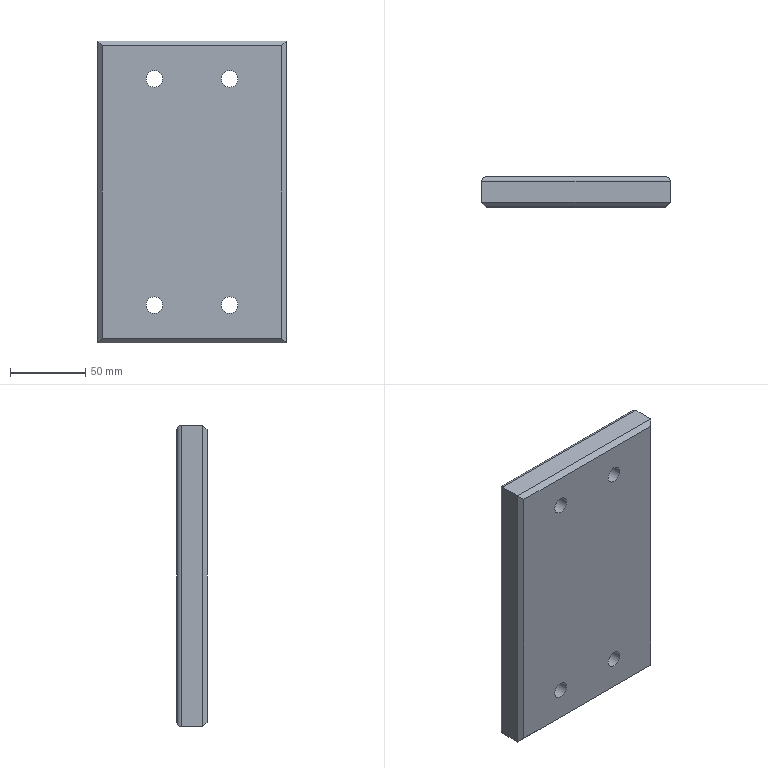Part | NX | features solid 2 | 1 solid | 26 faces | box 125 x 20 x 200 mm | volume 481280 mm3 | plane 14 | cylinder 12 | commonest cylinder face diameters 6 x4 11 x4 17.5 x4
STEP:
#1=CARTESIAN_POINT('',(-972.5,528.,-185.));
#2=VERTEX_POINT('',#1);
#3=CARTESIAN_POINT('',(-972.5,542.,-185.));
#4=VERTEX_POINT('',#3);
#5=CARTESIAN_POINT('',(-972.5,525.,-185.));
#6=DIRECTION('',(0.,1.,0.));
#7=VECTOR('',#6,1000.);
#8=LINE('',#5,#7);
#9=EDGE_CURVE('',#2,#4,#8,.T.);
#10=ORIENTED_EDGE('',*,*,#9,.F.);
#11=CARTESIAN_POINT('',(-1097.5,528.,-185.));
#12=VERTEX_POINT('',#11);
#13=CARTESIAN_POINT('',(-1097.5,528.,-185.));
#14=DIRECTION('',(-1.,0.,0.));
#15=VECTOR('',#14,1000.);
#16=LINE('',#13,#15);
#17=EDGE_CURVE('',#2,#12,#16,.T.);
#18=ORIENTED_EDGE('',*,*,#17,.T.);
#19=CARTESIAN_POINT('',(-1097.5,542.,-185.));
#20=VERTEX_POINT('',#19);
#21=CARTESIAN_POINT('',(-1097.5,525.,-185.));
#22=DIRECTION('',(0.,1.,0.));
#23=VECTOR('',#22,1000.);
#24=LINE('',#21,#23);
#25=EDGE_CURVE('',#12,#20,#24,.T.);
#26=ORIENTED_EDGE('',*,*,#25,.T.);
#27=CARTESIAN_POINT('',(-972.5,542.,-185.));
#28=DIRECTION('',(1.,0.,0.));
#29=VECTOR('',#28,1000.);
#30=LINE('',#27,#29);
#31=EDGE_CURVE('',#20,#4,#30,.T.);
#32=ORIENTED_EDGE('',*,*,#31,.T.);
#33=EDGE_LOOP('',(#10,#18,#26,#32));
#34=FACE_BOUND('',#33,.T.);
#35=CARTESIAN_POINT('',(-1097.5,525.,-185.));
#36=DIRECTION('',(0.,0.,1.));
#37=DIRECTION('',(-1.,0.,0.));
#38=AXIS2_PLACEMENT_3D('',#35,#36,#37);
#39=PLANE('',#38);
#40=ADVANCED_FACE('',(#34),#39,.F.);
#41=CARTESIAN_POINT('',(-972.5,528.,15.));
#42=VERTEX_POINT('',#41);
#43=CARTESIAN_POINT('',(-972.5,542.,15.));
#44=VERTEX_POINT('',#43);
#45=CARTESIAN_POINT('',(-972.5,525.,15.));
#46=DIRECTION('',(0.,1.,0.));
#47=VECTOR('',#46,1000.);
#48=LINE('',#45,#47);
#49=EDGE_CURVE('',#42,#44,#48,.T.);
#50=ORIENTED_EDGE('',*,*,#49,.F.);
#51=CARTESIAN_POINT('',(-972.5,528.,-185.));
#52=DIRECTION('',(0.,0.,-1.));
#53=VECTOR('',#52,1000.);
#54=LINE('',#51,#53);
#55=EDGE_CURVE('',#42,#2,#54,.T.);
#56=ORIENTED_EDGE('',*,*,#55,.T.);
#57=ORIENTED_EDGE('',*,*,#9,.T.);
#58=CARTESIAN_POINT('',(-972.5,542.,15.));
#59=DIRECTION('',(0.,0.,1.));
#60=VECTOR('',#59,1000.);
#61=LINE('',#58,#60);
#62=EDGE_CURVE('',#4,#44,#61,.T.);
#63=ORIENTED_EDGE('',*,*,#62,.T.);
#64=EDGE_LOOP('',(#50,#56,#57,#63));
#65=FACE_BOUND('',#64,.T.);
#66=CARTESIAN_POINT('',(-972.5,525.,-185.));
#67=DIRECTION('',(-1.,0.,0.));
#68=DIRECTION('',(0.,0.,-1.));
#69=AXIS2_PLACEMENT_3D('',#66,#67,#68);
#70=PLANE('',#69);
#71=ADVANCED_FACE('',(#65),#70,.F.);
#72=CARTESIAN_POINT('',(-1097.5,528.,15.));
#73=VERTEX_POINT('',#72);
#74=CARTESIAN_POINT('',(-1097.5,542.,15.));
#75=VERTEX_POINT('',#74);
#76=CARTESIAN_POINT('',(-1097.5,525.,15.));
#77=DIRECTION('',(0.,1.,0.));
#78=VECTOR('',#77,1000.);
#79=LINE('',#76,#78);
#80=EDGE_CURVE('',#73,#75,#79,.T.);
#81=ORIENTED_EDGE('',*,*,#80,.F.);
#82=CARTESIAN_POINT('',(-972.5,528.,15.));
#83=DIRECTION('',(1.,0.,0.));
#84=VECTOR('',#83,1000.);
#85=LINE('',#82,#84);
#86=EDGE_CURVE('',#73,#42,#85,.T.);
#87=ORIENTED_EDGE('',*,*,#86,.T.);
#88=ORIENTED_EDGE('',*,*,#49,.T.);
#89=CARTESIAN_POINT('',(-1097.5,542.,15.));
#90=DIRECTION('',(-1.,0.,0.));
#91=VECTOR('',#90,1000.);
#92=LINE('',#89,#91);
#93=EDGE_CURVE('',#44,#75,#92,.T.);
#94=ORIENTED_EDGE('',*,*,#93,.T.);
#95=EDGE_LOOP('',(#81,#87,#88,#94));
#96=FACE_BOUND('',#95,.T.);
#97=CARTESIAN_POINT('',(-972.5,525.,15.));
#98=DIRECTION('',(0.,0.,-1.));
#99=DIRECTION('',(0.,-1.,0.));
#100=AXIS2_PLACEMENT_3D('',#97,#98,#99);
#101=PLANE('',#100);
#102=ADVANCED_FACE('',(#96),#101,.F.);
#103=ORIENTED_EDGE('',*,*,#25,.F.);
#104=CARTESIAN_POINT('',(-1097.5,528.,15.));
#105=DIRECTION('',(0.,0.,1.));
#106=VECTOR('',#105,1000.);
#107=LINE('',#104,#106);
#108=EDGE_CURVE('',#12,#73,#107,.T.);
#109=ORIENTED_EDGE('',*,*,#108,.T.);
#110=ORIENTED_EDGE('',*,*,#80,.T.);
#111=CARTESIAN_POINT('',(-1097.5,542.,-185.));
#112=DIRECTION('',(0.,0.,-1.));
#113=VECTOR('',#112,1000.);
#114=LINE('',#111,#113);
#115=EDGE_CURVE('',#75,#20,#114,.T.);
#116=ORIENTED_EDGE('',*,*,#115,.T.);
#117=EDGE_LOOP('',(#103,#109,#110,#116));
#118=FACE_BOUND('',#117,.T.);
#119=CARTESIAN_POINT('',(-1097.5,525.,15.));
#120=DIRECTION('',(1.,0.,0.));
#121=DIRECTION('',(0.,0.,1.));
#122=AXIS2_PLACEMENT_3D('',#119,#120,#121);
#123=PLANE('',#122);
#124=ADVANCED_FACE('',(#118),#123,.F.);
#125=CARTESIAN_POINT('',(-975.5,525.,-182.));
#126=VERTEX_POINT('',#125);
#127=CARTESIAN_POINT('',(-975.5,525.,12.));
#128=VERTEX_POINT('',#127);
#129=CARTESIAN_POINT('',(-975.5,525.,-185.));
#130=DIRECTION('',(0.,0.,1.));
#131=VECTOR('',#130,1000.);
#132=LINE('',#129,#131);
#133=EDGE_CURVE('',#126,#128,#132,.T.);
#134=ORIENTED_EDGE('',*,*,#133,.T.);
#135=CARTESIAN_POINT('',(-1094.5,525.,12.));
#136=VERTEX_POINT('',#135);
#137=CARTESIAN_POINT('',(-1097.5,525.,12.));
#138=DIRECTION('',(-1.,0.,0.));
#139=VECTOR('',#138,1000.);
#140=LINE('',#137,#139);
#141=EDGE_CURVE('',#128,#136,#140,.T.);
#142=ORIENTED_EDGE('',*,*,#141,.T.);
#143=CARTESIAN_POINT('',(-1094.5,525.,-182.));
#144=VERTEX_POINT('',#143);
#145=CARTESIAN_POINT('',(-1094.5,525.,-185.));
#146=DIRECTION('',(0.,0.,-1.));
#147=VECTOR('',#146,1000.);
#148=LINE('',#145,#147);
#149=EDGE_CURVE('',#136,#144,#148,.T.);
#150=ORIENTED_EDGE('',*,*,#149,.T.);
#151=CARTESIAN_POINT('',(-1097.5,525.,-182.));
#152=DIRECTION('',(1.,0.,0.));
#153=VECTOR('',#152,1000.);
#154=LINE('',#151,#153);
#155=EDGE_CURVE('',#144,#126,#154,.T.);
#156=ORIENTED_EDGE('',*,*,#155,.T.);
#157=EDGE_LOOP('',(#134,#142,#150,#156));
#158=FACE_BOUND('',#157,.T.);
#159=CARTESIAN_POINT('',(-1010.,525.,-15.5));
#160=VERTEX_POINT('',#159);
#161=CARTESIAN_POINT('',(-1010.,525.,-10.));
#162=DIRECTION('',(0.,1.,0.));
#163=DIRECTION('',(0.,0.,-1.));
#164=AXIS2_PLACEMENT_3D('',#161,#162,#163);
#165=CIRCLE('',#164,5.5);
#166=EDGE_CURVE('',#160,#160,#165,.T.);
#167=ORIENTED_EDGE('',*,*,#166,.T.);
#168=EDGE_LOOP('',(#167));
#169=FACE_BOUND('',#168,.T.);
#170=CARTESIAN_POINT('',(-1060.,525.,-15.5));
#171=VERTEX_POINT('',#170);
#172=CARTESIAN_POINT('',(-1060.,525.,-10.));
#173=DIRECTION('',(0.,1.,0.));
#174=DIRECTION('',(0.,0.,-1.));
#175=AXIS2_PLACEMENT_3D('',#172,#173,#174);
#176=CIRCLE('',#175,5.5);
#177=EDGE_CURVE('',#171,#171,#176,.T.);
#178=ORIENTED_EDGE('',*,*,#177,.T.);
#179=EDGE_LOOP('',(#178));
#180=FACE_BOUND('',#179,.T.);
#181=CARTESIAN_POINT('',(-1010.,525.,-165.5));
#182=VERTEX_POINT('',#181);
#183=CARTESIAN_POINT('',(-1010.,525.,-160.));
#184=DIRECTION('',(0.,1.,0.));
#185=DIRECTION('',(0.,0.,-1.));
#186=AXIS2_PLACEMENT_3D('',#183,#184,#185);
#187=CIRCLE('',#186,5.5);
#188=EDGE_CURVE('',#182,#182,#187,.T.);
#189=ORIENTED_EDGE('',*,*,#188,.T.);
#190=EDGE_LOOP('',(#189));
#191=FACE_BOUND('',#190,.T.);
#192=CARTESIAN_POINT('',(-1060.,525.,-165.5));
#193=VERTEX_POINT('',#192);
#194=CARTESIAN_POINT('',(-1060.,525.,-160.));
#195=DIRECTION('',(0.,1.,0.));
#196=DIRECTION('',(0.,0.,-1.));
#197=AXIS2_PLACEMENT_3D('',#194,#195,#196);
#198=CIRCLE('',#197,5.5);
#199=EDGE_CURVE('',#193,#193,#198,.T.);
#200=ORIENTED_EDGE('',*,*,#199,.T.);
#201=EDGE_LOOP('',(#200));
#202=FACE_BOUND('',#201,.T.);
#203=CARTESIAN_POINT('',(-1097.5,525.,-185.));
#204=DIRECTION('',(0.,1.,0.));
#205=DIRECTION('',(0.,0.,-1.));
#206=AXIS2_PLACEMENT_3D('',#203,#204,#205);
#207=PLANE('',#206);
#208=ADVANCED_FACE('',(#158,#169,#180,#191,#202),#207,.F.);
#209=CARTESIAN_POINT('',(-975.5,545.,-182.));
#210=VERTEX_POINT('',#209);
#211=CARTESIAN_POINT('',(-1094.5,545.,-182.));
#212=VERTEX_POINT('',#211);
#213=CARTESIAN_POINT('',(-1097.5,545.,-182.));
#214=DIRECTION('',(1.,0.,0.));
#215=VECTOR('',#214,1000.);
#216=LINE('',#213,#215);
#217=EDGE_CURVE('',#210,#212,#216,.F.);
#218=ORIENTED_EDGE('',*,*,#217,.T.);
#219=CARTESIAN_POINT('',(-1094.5,545.,12.));
#220=VERTEX_POINT('',#219);
#221=CARTESIAN_POINT('',(-1094.5,545.,15.));
#222=DIRECTION('',(0.,0.,-1.));
#223=VECTOR('',#222,1000.);
#224=LINE('',#221,#223);
#225=EDGE_CURVE('',#212,#220,#224,.F.);
#226=ORIENTED_EDGE('',*,*,#225,.T.);
#227=CARTESIAN_POINT('',(-975.5,545.,12.));
#228=VERTEX_POINT('',#227);
#229=CARTESIAN_POINT('',(-972.5,545.,12.));
#230=DIRECTION('',(-1.,0.,0.));
#231=VECTOR('',#230,1000.);
#232=LINE('',#229,#231);
#233=EDGE_CURVE('',#220,#228,#232,.F.);
#234=ORIENTED_EDGE('',*,*,#233,.T.);
#235=CARTESIAN_POINT('',(-975.5,545.,-185.));
#236=DIRECTION('',(0.,0.,1.));
#237=VECTOR('',#236,1000.);
#238=LINE('',#235,#237);
#239=EDGE_CURVE('',#228,#210,#238,.F.);
#240=ORIENTED_EDGE('',*,*,#239,.T.);
#241=EDGE_LOOP('',(#218,#226,#234,#240));
#242=FACE_BOUND('',#241,.T.);
#243=CARTESIAN_POINT('',(-1010.,545.,-1.25));
#244=VERTEX_POINT('',#243);
#245=CARTESIAN_POINT('',(-1010.,545.,-10.));
#246=DIRECTION('',(0.,-1.,0.));
#247=DIRECTION('',(0.,0.,1.));
#248=AXIS2_PLACEMENT_3D('',#245,#246,#247);
#249=CIRCLE('',#248,8.75);
#250=EDGE_CURVE('',#244,#244,#249,.T.);
#251=ORIENTED_EDGE('',*,*,#250,.T.);
#252=EDGE_LOOP('',(#251));
#253=FACE_BOUND('',#252,.T.);
#254=CARTESIAN_POINT('',(-1060.,545.,-1.25));
#255=VERTEX_POINT('',#254);
#256=CARTESIAN_POINT('',(-1060.,545.,-10.));
#257=DIRECTION('',(0.,-1.,0.));
#258=DIRECTION('',(0.,0.,1.));
#259=AXIS2_PLACEMENT_3D('',#256,#257,#258);
#260=CIRCLE('',#259,8.75);
#261=EDGE_CURVE('',#255,#255,#260,.T.);
#262=ORIENTED_EDGE('',*,*,#261,.T.);
#263=EDGE_LOOP('',(#262));
#264=FACE_BOUND('',#263,.T.);
#265=CARTESIAN_POINT('',(-1010.,545.,-151.25));
#266=VERTEX_POINT('',#265);
#267=CARTESIAN_POINT('',(-1010.,545.,-160.));
#268=DIRECTION('',(0.,-1.,0.));
#269=DIRECTION('',(0.,0.,1.));
#270=AXIS2_PLACEMENT_3D('',#267,#268,#269);
#271=CIRCLE('',#270,8.75);
#272=EDGE_CURVE('',#266,#266,#271,.T.);
#273=ORIENTED_EDGE('',*,*,#272,.T.);
#274=EDGE_LOOP('',(#273));
#275=FACE_BOUND('',#274,.T.);
#276=CARTESIAN_POINT('',(-1060.,545.,-151.25));
#277=VERTEX_POINT('',#276);
#278=CARTESIAN_POINT('',(-1060.,545.,-160.));
#279=DIRECTION('',(0.,-1.,0.));
#280=DIRECTION('',(0.,0.,1.));
#281=AXIS2_PLACEMENT_3D('',#278,#279,#280);
#282=CIRCLE('',#281,8.75);
#283=EDGE_CURVE('',#277,#277,#282,.T.);
#284=ORIENTED_EDGE('',*,*,#283,.T.);
#285=EDGE_LOOP('',(#284));
#286=FACE_BOUND('',#285,.T.);
#287=CARTESIAN_POINT('',(-1097.5,545.,-185.));
#288=DIRECTION('',(0.,1.,0.));
#289=DIRECTION('',(0.,0.,-1.));
#290=AXIS2_PLACEMENT_3D('',#287,#288,#289);
#291=PLANE('',#290);
#292=ADVANCED_FACE('',(#242,#253,#264,#275,#286),#291,.T.);
#293=CARTESIAN_POINT('',(-1060.,533.,-154.5));
#294=VERTEX_POINT('',#293);
#295=CARTESIAN_POINT('',(-1060.,533.,-160.));
#296=DIRECTION('',(0.,-1.,0.));
#297=DIRECTION('',(0.,0.,1.));
#298=AXIS2_PLACEMENT_3D('',#295,#296,#297);
#299=CIRCLE('',#298,5.5);
#300=EDGE_CURVE('',#294,#294,#299,.T.);
#301=ORIENTED_EDGE('',*,*,#300,.F.);
#302=EDGE_LOOP('',(#301));
#303=FACE_BOUND('',#302,.T.);
#304=ORIENTED_EDGE('',*,*,#199,.F.);
#305=EDGE_LOOP('',(#304));
#306=FACE_BOUND('',#305,.T.);
#307=CARTESIAN_POINT('',(-1060.,495.,-160.));
#308=DIRECTION('',(0.,-1.,0.));
#309=DIRECTION('',(0.,0.,1.));
#310=AXIS2_PLACEMENT_3D('',#307,#308,#309);
#311=CYLINDRICAL_SURFACE('',#310,5.5);
#312=ADVANCED_FACE('',(#303,#306),#311,.F.);
#313=ORIENTED_EDGE('',*,*,#300,.T.);
#314=EDGE_LOOP('',(#313));
#315=FACE_BOUND('',#314,.T.);
#316=CARTESIAN_POINT('',(-1060.,533.,-151.25));
#317=VERTEX_POINT('',#316);
#318=CARTESIAN_POINT('',(-1060.,533.,-160.));
#319=DIRECTION('',(0.,-1.,0.));
#320=DIRECTION('',(0.,0.,1.));
#321=AXIS2_PLACEMENT_3D('',#318,#319,#320);
#322=CIRCLE('',#321,8.75);
#323=EDGE_CURVE('',#317,#317,#322,.T.);
#324=ORIENTED_EDGE('',*,*,#323,.F.);
#325=EDGE_LOOP('',(#324));
#326=FACE_BOUND('',#325,.T.);
#327=CARTESIAN_POINT('',(-1060.,533.,-160.));
#328=DIRECTION('',(0.,-1.,0.));
#329=DIRECTION('',(0.,0.,1.));
#330=AXIS2_PLACEMENT_3D('',#327,#328,#329);
#331=PLANE('',#330);
#332=ADVANCED_FACE('',(#315,#326),#331,.F.);
#333=ORIENTED_EDGE('',*,*,#323,.T.);
#334=EDGE_LOOP('',(#333));
#335=FACE_BOUND('',#334,.T.);
#336=ORIENTED_EDGE('',*,*,#283,.F.);
#337=EDGE_LOOP('',(#336));
#338=FACE_BOUND('',#337,.T.);
#339=CARTESIAN_POINT('',(-1060.,545.,-160.));
#340=DIRECTION('',(0.,-1.,0.));
#341=DIRECTION('',(0.,0.,1.));
#342=AXIS2_PLACEMENT_3D('',#339,#340,#341);
#343=CYLINDRICAL_SURFACE('',#342,8.75);
#344=ADVANCED_FACE('',(#335,#338),#343,.F.);
#345=CARTESIAN_POINT('',(-1010.,533.,-154.5));
#346=VERTEX_POINT('',#345);
#347=CARTESIAN_POINT('',(-1010.,533.,-160.));
#348=DIRECTION('',(0.,-1.,0.));
#349=DIRECTION('',(0.,0.,1.));
#350=AXIS2_PLACEMENT_3D('',#347,#348,#349);
#351=CIRCLE('',#350,5.5);
#352=EDGE_CURVE('',#346,#346,#351,.T.);
#353=ORIENTED_EDGE('',*,*,#352,.F.);
#354=EDGE_LOOP('',(#353));
#355=FACE_BOUND('',#354,.T.);
#356=ORIENTED_EDGE('',*,*,#188,.F.);
#357=EDGE_LOOP('',(#356));
#358=FACE_BOUND('',#357,.T.);
#359=CARTESIAN_POINT('',(-1010.,495.,-160.));
#360=DIRECTION('',(0.,-1.,0.));
#361=DIRECTION('',(0.,0.,1.));
#362=AXIS2_PLACEMENT_3D('',#359,#360,#361);
#363=CYLINDRICAL_SURFACE('',#362,5.5);
#364=ADVANCED_FACE('',(#355,#358),#363,.F.);
#365=ORIENTED_EDGE('',*,*,#352,.T.);
#366=EDGE_LOOP('',(#365));
#367=FACE_BOUND('',#366,.T.);
#368=CARTESIAN_POINT('',(-1010.,533.,-151.25));
#369=VERTEX_POINT('',#368);
#370=CARTESIAN_POINT('',(-1010.,533.,-160.));
#371=DIRECTION('',(0.,-1.,0.));
#372=DIRECTION('',(0.,0.,1.));
#373=AXIS2_PLACEMENT_3D('',#370,#371,#372);
#374=CIRCLE('',#373,8.75);
#375=EDGE_CURVE('',#369,#369,#374,.T.);
#376=ORIENTED_EDGE('',*,*,#375,.F.);
#377=EDGE_LOOP('',(#376));
#378=FACE_BOUND('',#377,.T.);
#379=CARTESIAN_POINT('',(-1010.,533.,-160.));
#380=DIRECTION('',(0.,-1.,0.));
#381=DIRECTION('',(0.,0.,1.));
#382=AXIS2_PLACEMENT_3D('',#379,#380,#381);
#383=PLANE('',#382);
#384=ADVANCED_FACE('',(#367,#378),#383,.F.);
#385=ORIENTED_EDGE('',*,*,#375,.T.);
#386=EDGE_LOOP('',(#385));
#387=FACE_BOUND('',#386,.T.);
#388=ORIENTED_EDGE('',*,*,#272,.F.);
#389=EDGE_LOOP('',(#388));
#390=FACE_BOUND('',#389,.T.);
#391=CARTESIAN_POINT('',(-1010.,545.,-160.));
#392=DIRECTION('',(0.,-1.,0.));
#393=DIRECTION('',(0.,0.,1.));
#394=AXIS2_PLACEMENT_3D('',#391,#392,#393);
#395=CYLINDRICAL_SURFACE('',#394,8.75);
#396=ADVANCED_FACE('',(#387,#390),#395,.F.);
#397=CARTESIAN_POINT('',(-1060.,533.,-4.5));
#398=VERTEX_POINT('',#397);
#399=CARTESIAN_POINT('',(-1060.,533.,-10.));
#400=DIRECTION('',(0.,-1.,0.));
#401=DIRECTION('',(0.,0.,1.));
#402=AXIS2_PLACEMENT_3D('',#399,#400,#401);
#403=CIRCLE('',#402,5.5);
#404=EDGE_CURVE('',#398,#398,#403,.T.);
#405=ORIENTED_EDGE('',*,*,#404,.F.);
#406=EDGE_LOOP('',(#405));
#407=FACE_BOUND('',#406,.T.);
#408=ORIENTED_EDGE('',*,*,#177,.F.);
#409=EDGE_LOOP('',(#408));
#410=FACE_BOUND('',#409,.T.);
#411=CARTESIAN_POINT('',(-1060.,495.,-10.));
#412=DIRECTION('',(0.,-1.,0.));
#413=DIRECTION('',(0.,0.,1.));
#414=AXIS2_PLACEMENT_3D('',#411,#412,#413);
#415=CYLINDRICAL_SURFACE('',#414,5.5);
#416=ADVANCED_FACE('',(#407,#410),#415,.F.);
#417=ORIENTED_EDGE('',*,*,#404,.T.);
#418=EDGE_LOOP('',(#417));
#419=FACE_BOUND('',#418,.T.);
#420=CARTESIAN_POINT('',(-1060.,533.,-1.25));
#421=VERTEX_POINT('',#420);
#422=CARTESIAN_POINT('',(-1060.,533.,-10.));
#423=DIRECTION('',(0.,-1.,0.));
#424=DIRECTION('',(0.,0.,1.));
#425=AXIS2_PLACEMENT_3D('',#422,#423,#424);
#426=CIRCLE('',#425,8.75);
#427=EDGE_CURVE('',#421,#421,#426,.T.);
#428=ORIENTED_EDGE('',*,*,#427,.F.);
#429=EDGE_LOOP('',(#428));
#430=FACE_BOUND('',#429,.T.);
#431=CARTESIAN_POINT('',(-1060.,533.,-10.));
#432=DIRECTION('',(0.,-1.,0.));
#433=DIRECTION('',(0.,0.,1.));
#434=AXIS2_PLACEMENT_3D('',#431,#432,#433);
#435=PLANE('',#434);
#436=ADVANCED_FACE('',(#419,#430),#435,.F.);
#437=ORIENTED_EDGE('',*,*,#427,.T.);
#438=EDGE_LOOP('',(#437));
#439=FACE_BOUND('',#438,.T.);
#440=ORIENTED_EDGE('',*,*,#261,.F.);
#441=EDGE_LOOP('',(#440));
#442=FACE_BOUND('',#441,.T.);
#443=CARTESIAN_POINT('',(-1060.,545.,-10.));
#444=DIRECTION('',(0.,-1.,0.));
#445=DIRECTION('',(0.,0.,1.));
#446=AXIS2_PLACEMENT_3D('',#443,#444,#445);
#447=CYLINDRICAL_SURFACE('',#446,8.75);
#448=ADVANCED_FACE('',(#439,#442),#447,.F.);
#449=CARTESIAN_POINT('',(-1010.,533.,-4.5));
#450=VERTEX_POINT('',#449);
#451=CARTESIAN_POINT('',(-1010.,533.,-10.));
#452=DIRECTION('',(0.,-1.,0.));
#453=DIRECTION('',(0.,0.,1.));
#454=AXIS2_PLACEMENT_3D('',#451,#452,#453);
#455=CIRCLE('',#454,5.5);
#456=EDGE_CURVE('',#450,#450,#455,.T.);
#457=ORIENTED_EDGE('',*,*,#456,.F.);
#458=EDGE_LOOP('',(#457));
#459=FACE_BOUND('',#458,.T.);
#460=ORIENTED_EDGE('',*,*,#166,.F.);
#461=EDGE_LOOP('',(#460));
#462=FACE_BOUND('',#461,.T.);
#463=CARTESIAN_POINT('',(-1010.,495.,-10.));
#464=DIRECTION('',(0.,-1.,0.));
#465=DIRECTION('',(0.,0.,1.));
#466=AXIS2_PLACEMENT_3D('',#463,#464,#465);
#467=CYLINDRICAL_SURFACE('',#466,5.5);
#468=ADVANCED_FACE('',(#459,#462),#467,.F.);
#469=ORIENTED_EDGE('',*,*,#456,.T.);
#470=EDGE_LOOP('',(#469));
#471=FACE_BOUND('',#470,.T.);
#472=CARTESIAN_POINT('',(-1010.,533.,-1.25));
#473=VERTEX_POINT('',#472);
#474=CARTESIAN_POINT('',(-1010.,533.,-10.));
#475=DIRECTION('',(0.,-1.,0.));
#476=DIRECTION('',(0.,0.,1.));
#477=AXIS2_PLACEMENT_3D('',#474,#475,#476);
#478=CIRCLE('',#477,8.75);
#479=EDGE_CURVE('',#473,#473,#478,.T.);
#480=ORIENTED_EDGE('',*,*,#479,.F.);
#481=EDGE_LOOP('',(#480));
#482=FACE_BOUND('',#481,.T.);
#483=CARTESIAN_POINT('',(-1010.,533.,-10.));
#484=DIRECTION('',(0.,-1.,0.));
#485=DIRECTION('',(0.,0.,1.));
#486=AXIS2_PLACEMENT_3D('',#483,#484,#485);
#487=PLANE('',#486);
#488=ADVANCED_FACE('',(#471,#482),#487,.F.);
#489=ORIENTED_EDGE('',*,*,#479,.T.);
#490=EDGE_LOOP('',(#489));
#491=FACE_BOUND('',#490,.T.);
#492=ORIENTED_EDGE('',*,*,#250,.F.);
#493=EDGE_LOOP('',(#492));
#494=FACE_BOUND('',#493,.T.);
#495=CARTESIAN_POINT('',(-1010.,545.,-10.));
#496=DIRECTION('',(0.,-1.,0.));
#497=DIRECTION('',(0.,0.,1.));
#498=AXIS2_PLACEMENT_3D('',#495,#496,#497);
#499=CYLINDRICAL_SURFACE('',#498,8.75);
#500=ADVANCED_FACE('',(#491,#494),#499,.F.);
#501=CARTESIAN_POINT('',(-975.5,542.,-182.));
#502=DIRECTION('',(-0.7071,0.,-0.7071));
#503=DIRECTION('',(-0.7071,0.,0.7071));
#504=AXIS2_PLACEMENT_3D('',#501,#502,#503);
#505=ELLIPSE('',#504,4.243,3.);
#506=EDGE_CURVE('',#210,#4,#505,.T.);
#507=ORIENTED_EDGE('',*,*,#506,.F.);
#508=ORIENTED_EDGE('',*,*,#239,.F.);
#509=CARTESIAN_POINT('',(-975.5,542.,12.));
#510=DIRECTION('',(0.7071,0.,-0.7071));
#511=DIRECTION('',(-0.7071,0.,-0.7071));
#512=AXIS2_PLACEMENT_3D('',#509,#510,#511);
#513=ELLIPSE('',#512,4.243,3.);
#514=EDGE_CURVE('',#44,#228,#513,.F.);
#515=ORIENTED_EDGE('',*,*,#514,.F.);
#516=ORIENTED_EDGE('',*,*,#62,.F.);
#517=EDGE_LOOP('',(#507,#508,#515,#516));
#518=FACE_BOUND('',#517,.T.);
#519=CARTESIAN_POINT('',(-975.5,542.,-185.));
#520=DIRECTION('',(0.,0.,-1.));
#521=DIRECTION('',(1.,0.,0.));
#522=AXIS2_PLACEMENT_3D('',#519,#520,#521);
#523=CYLINDRICAL_SURFACE('',#522,3.);
#524=ADVANCED_FACE('',(#518),#523,.T.);
#525=ORIENTED_EDGE('',*,*,#514,.T.);
#526=ORIENTED_EDGE('',*,*,#233,.F.);
#527=CARTESIAN_POINT('',(-1094.5,542.,12.));
#528=DIRECTION('',(0.7071,0.,0.7071));
#529=DIRECTION('',(0.7071,0.,-0.7071));
#530=AXIS2_PLACEMENT_3D('',#527,#528,#529);
#531=ELLIPSE('',#530,4.243,3.);
#532=EDGE_CURVE('',#75,#220,#531,.F.);
#533=ORIENTED_EDGE('',*,*,#532,.F.);
#534=ORIENTED_EDGE('',*,*,#93,.F.);
#535=EDGE_LOOP('',(#525,#526,#533,#534));
#536=FACE_BOUND('',#535,.T.);
#537=CARTESIAN_POINT('',(-972.5,542.,12.));
#538=DIRECTION('',(1.,0.,0.));
#539=DIRECTION('',(0.,1.,0.));
#540=AXIS2_PLACEMENT_3D('',#537,#538,#539);
#541=CYLINDRICAL_SURFACE('',#540,3.);
#542=ADVANCED_FACE('',(#536),#541,.T.);
#543=ORIENTED_EDGE('',*,*,#506,.T.);
#544=ORIENTED_EDGE('',*,*,#31,.F.);
#545=CARTESIAN_POINT('',(-1094.5,542.,-182.));
#546=DIRECTION('',(-0.7071,0.,0.7071));
#547=DIRECTION('',(-0.7071,0.,-0.7071));
#548=AXIS2_PLACEMENT_3D('',#545,#546,#547);
#549=ELLIPSE('',#548,4.243,3.);
#550=EDGE_CURVE('',#212,#20,#549,.T.);
#551=ORIENTED_EDGE('',*,*,#550,.F.);
#552=ORIENTED_EDGE('',*,*,#217,.F.);
#553=EDGE_LOOP('',(#543,#544,#551,#552));
#554=FACE_BOUND('',#553,.T.);
#555=CARTESIAN_POINT('',(-1097.5,542.,-182.));
#556=DIRECTION('',(-1.,0.,0.));
#557=DIRECTION('',(0.,0.,-1.));
#558=AXIS2_PLACEMENT_3D('',#555,#556,#557);
#559=CYLINDRICAL_SURFACE('',#558,3.);
#560=ADVANCED_FACE('',(#554),#559,.T.);
#561=ORIENTED_EDGE('',*,*,#532,.T.);
#562=ORIENTED_EDGE('',*,*,#225,.F.);
#563=ORIENTED_EDGE('',*,*,#550,.T.);
#564=ORIENTED_EDGE('',*,*,#115,.F.);
#565=EDGE_LOOP('',(#561,#562,#563,#564));
#566=FACE_BOUND('',#565,.T.);
#567=CARTESIAN_POINT('',(-1094.5,542.,15.));
#568=DIRECTION('',(0.,0.,1.));
#569=DIRECTION('',(-1.,0.,0.));
#570=AXIS2_PLACEMENT_3D('',#567,#568,#569);
#571=CYLINDRICAL_SURFACE('',#570,3.);
#572=ADVANCED_FACE('',(#566),#571,.T.);
#573=CARTESIAN_POINT('',(-1095.5,526.,-183.));
#574=DIRECTION('',(0.5774,-0.5774,0.5774));
#575=VECTOR('',#574,1000.);
#576=LINE('',#573,#575);
#577=EDGE_CURVE('',#12,#144,#576,.T.);
#578=ORIENTED_EDGE('',*,*,#577,.F.);
#579=ORIENTED_EDGE('',*,*,#17,.F.);
#580=CARTESIAN_POINT('',(-1016.167,484.333,-141.333));
#581=DIRECTION('',(-0.5774,-0.5774,0.5774));
#582=VECTOR('',#581,1000.);
#583=LINE('',#580,#582);
#584=EDGE_CURVE('',#126,#2,#583,.F.);
#585=ORIENTED_EDGE('',*,*,#584,.F.);
#586=ORIENTED_EDGE('',*,*,#155,.F.);
#587=EDGE_LOOP('',(#578,#579,#585,#586));
#588=FACE_BOUND('',#587,.T.);
#589=CARTESIAN_POINT('',(-1097.5,525.,-182.));
#590=DIRECTION('',(0.,0.7071,0.7071));
#591=DIRECTION('',(0.,0.7071,-0.7071));
#592=AXIS2_PLACEMENT_3D('',#589,#590,#591);
#593=PLANE('',#592);
#594=ADVANCED_FACE('',(#588),#593,.F.);
#595=ORIENTED_EDGE('',*,*,#584,.T.);
#596=ORIENTED_EDGE('',*,*,#55,.F.);
#597=CARTESIAN_POINT('',(-1041.167,459.333,-53.667));
#598=DIRECTION('',(-0.5774,-0.5774,-0.5774));
#599=VECTOR('',#598,1000.);
#600=LINE('',#597,#599);
#601=EDGE_CURVE('',#128,#42,#600,.F.);
#602=ORIENTED_EDGE('',*,*,#601,.F.);
#603=ORIENTED_EDGE('',*,*,#133,.F.);
#604=EDGE_LOOP('',(#595,#596,#602,#603));
#605=FACE_BOUND('',#604,.T.);
#606=CARTESIAN_POINT('',(-975.5,525.,-185.));
#607=DIRECTION('',(-0.7071,0.7071,0.));
#608=DIRECTION('',(-0.7071,-0.7071,0.));
#609=AXIS2_PLACEMENT_3D('',#606,#607,#608);
#610=PLANE('',#609);
#611=ADVANCED_FACE('',(#605),#610,.F.);
#612=ORIENTED_EDGE('',*,*,#577,.T.);
#613=ORIENTED_EDGE('',*,*,#149,.F.);
#614=CARTESIAN_POINT('',(-1028.833,459.333,-53.667));
#615=DIRECTION('',(-0.5774,0.5774,0.5774));
#616=VECTOR('',#615,1000.);
#617=LINE('',#614,#616);
#618=EDGE_CURVE('',#73,#136,#617,.F.);
#619=ORIENTED_EDGE('',*,*,#618,.F.);
#620=ORIENTED_EDGE('',*,*,#108,.F.);
#621=EDGE_LOOP('',(#612,#613,#619,#620));
#622=FACE_BOUND('',#621,.T.);
#623=CARTESIAN_POINT('',(-1094.5,525.,-185.));
#624=DIRECTION('',(0.7071,0.7071,0.));
#625=DIRECTION('',(-0.7071,0.7071,0.));
#626=AXIS2_PLACEMENT_3D('',#623,#624,#625);
#627=PLANE('',#626);
#628=ADVANCED_FACE('',(#622),#627,.F.);
#629=ORIENTED_EDGE('',*,*,#601,.T.);
#630=ORIENTED_EDGE('',*,*,#86,.F.);
#631=ORIENTED_EDGE('',*,*,#618,.T.);
#632=ORIENTED_EDGE('',*,*,#141,.F.);
#633=EDGE_LOOP('',(#629,#630,#631,#632));
#634=FACE_BOUND('',#633,.T.);
#635=CARTESIAN_POINT('',(-1097.5,525.,12.));
#636=DIRECTION('',(0.,0.7071,-0.7071));
#637=DIRECTION('',(0.,-0.7071,-0.7071));
#638=AXIS2_PLACEMENT_3D('',#635,#636,#637);
#639=PLANE('',#638);
#640=ADVANCED_FACE('',(#634),#639,.F.);
#641=CLOSED_SHELL('',(#40,#71,#102,#124,#208,#292,#312,#332,#344,#364,#384,#396,#416,#436,#448,#468,#488,#500,#524,#542,#560,#572,#594,#611,#628,#640));
#642=MANIFOLD_SOLID_BREP('',#641);
#643=(LENGTH_UNIT()NAMED_UNIT(*)SI_UNIT(.MILLI.,.METRE.));
#644=UNCERTAINTY_MEASURE_WITH_UNIT(LENGTH_MEASURE(0.00001),#643,'','');
#645=(NAMED_UNIT(*)PLANE_ANGLE_UNIT()SI_UNIT($,.RADIAN.));
#646=(NAMED_UNIT(*)SI_UNIT($,.STERADIAN.)SOLID_ANGLE_UNIT());
#647=(GEOMETRIC_REPRESENTATION_CONTEXT(3)GLOBAL_UNCERTAINTY_ASSIGNED_CONTEXT((#644))GLOBAL_UNIT_ASSIGNED_CONTEXT((#643,#645,#646))REPRESENTATION_CONTEXT('',''));
#648=ADVANCED_BREP_SHAPE_REPRESENTATION('',(#642),#647);